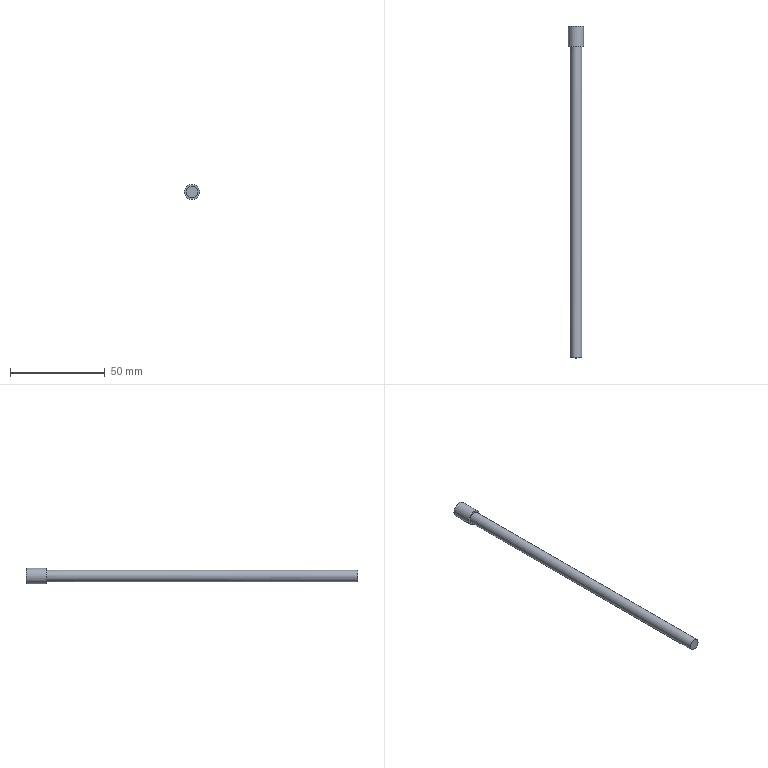Part | NX | features solid 2 | 1 solid | 5 faces | box 8 x 175 x 8 mm | volume 5190 mm3 | plane 3 | cylinder 2 | commonest cylinder face diameters 6 x1 8 x1
STEP:
#1=CARTESIAN_POINT('',(-39.,-65.,-52.));
#2=VERTEX_POINT('',#1);
#3=CARTESIAN_POINT('',(-42.,-65.,-52.));
#4=DIRECTION('',(0.,1.,0.));
#5=DIRECTION('',(1.,0.,0.));
#6=AXIS2_PLACEMENT_3D('',#3,#4,#5);
#7=CIRCLE('',#6,3.);
#8=EDGE_CURVE('',#2,#2,#7,.T.);
#9=ORIENTED_EDGE('',*,*,#8,.F.);
#10=EDGE_LOOP('',(#9));
#11=FACE_BOUND('',#10,.T.);
#12=CARTESIAN_POINT('',(-42.,-65.,-52.));
#13=DIRECTION('',(0.,-1.,0.));
#14=DIRECTION('',(0.,0.,-1.));
#15=AXIS2_PLACEMENT_3D('',#12,#13,#14);
#16=PLANE('',#15);
#17=ADVANCED_FACE('',(#11),#16,.T.);
#18=CARTESIAN_POINT('',(-42.,99.,-55.));
#19=VERTEX_POINT('',#18);
#20=CARTESIAN_POINT('',(-42.,99.,-52.));
#21=DIRECTION('',(0.,-1.,0.));
#22=DIRECTION('',(0.,0.,-1.));
#23=AXIS2_PLACEMENT_3D('',#20,#21,#22);
#24=CIRCLE('',#23,3.);
#25=EDGE_CURVE('',#19,#19,#24,.F.);
#26=ORIENTED_EDGE('',*,*,#25,.F.);
#27=EDGE_LOOP('',(#26));
#28=FACE_BOUND('',#27,.T.);
#29=ORIENTED_EDGE('',*,*,#8,.T.);
#30=EDGE_LOOP('',(#29));
#31=FACE_BOUND('',#30,.T.);
#32=CARTESIAN_POINT('',(-42.,110.,-52.));
#33=DIRECTION('',(0.,-1.,0.));
#34=DIRECTION('',(1.,0.,0.));
#35=AXIS2_PLACEMENT_3D('',#32,#33,#34);
#36=CYLINDRICAL_SURFACE('',#35,3.);
#37=ADVANCED_FACE('',(#28,#31),#36,.T.);
#38=ORIENTED_EDGE('',*,*,#25,.T.);
#39=EDGE_LOOP('',(#38));
#40=FACE_BOUND('',#39,.T.);
#41=CARTESIAN_POINT('',(-38.,99.,-52.));
#42=VERTEX_POINT('',#41);
#43=CARTESIAN_POINT('',(-42.,99.,-52.));
#44=DIRECTION('',(0.,1.,0.));
#45=DIRECTION('',(1.,0.,0.));
#46=AXIS2_PLACEMENT_3D('',#43,#44,#45);
#47=CIRCLE('',#46,4.);
#48=EDGE_CURVE('',#42,#42,#47,.T.);
#49=ORIENTED_EDGE('',*,*,#48,.F.);
#50=EDGE_LOOP('',(#49));
#51=FACE_BOUND('',#50,.T.);
#52=CARTESIAN_POINT('',(-42.,99.,-52.));
#53=DIRECTION('',(0.,-1.,0.));
#54=DIRECTION('',(0.,0.,-1.));
#55=AXIS2_PLACEMENT_3D('',#52,#53,#54);
#56=PLANE('',#55);
#57=ADVANCED_FACE('',(#40,#51),#56,.T.);
#58=ORIENTED_EDGE('',*,*,#48,.T.);
#59=EDGE_LOOP('',(#58));
#60=FACE_BOUND('',#59,.T.);
#61=CARTESIAN_POINT('',(-38.,110.,-52.));
#62=VERTEX_POINT('',#61);
#63=CARTESIAN_POINT('',(-42.,110.,-52.));
#64=DIRECTION('',(0.,-1.,0.));
#65=DIRECTION('',(1.,0.,0.));
#66=AXIS2_PLACEMENT_3D('',#63,#64,#65);
#67=CIRCLE('',#66,4.);
#68=EDGE_CURVE('',#62,#62,#67,.T.);
#69=ORIENTED_EDGE('',*,*,#68,.T.);
#70=EDGE_LOOP('',(#69));
#71=FACE_BOUND('',#70,.T.);
#72=CARTESIAN_POINT('',(-42.,110.,-52.));
#73=DIRECTION('',(0.,-1.,0.));
#74=DIRECTION('',(1.,0.,0.));
#75=AXIS2_PLACEMENT_3D('',#72,#73,#74);
#76=CYLINDRICAL_SURFACE('',#75,4.);
#77=ADVANCED_FACE('',(#60,#71),#76,.T.);
#78=ORIENTED_EDGE('',*,*,#68,.F.);
#79=EDGE_LOOP('',(#78));
#80=FACE_BOUND('',#79,.T.);
#81=CARTESIAN_POINT('',(-42.,110.,-52.));
#82=DIRECTION('',(0.,1.,0.));
#83=DIRECTION('',(0.,0.,1.));
#84=AXIS2_PLACEMENT_3D('',#81,#82,#83);
#85=PLANE('',#84);
#86=ADVANCED_FACE('',(#80),#85,.T.);
#87=CLOSED_SHELL('',(#17,#37,#57,#77,#86));
#88=MANIFOLD_SOLID_BREP('',#87);
#89=(LENGTH_UNIT()NAMED_UNIT(*)SI_UNIT(.MILLI.,.METRE.));
#90=UNCERTAINTY_MEASURE_WITH_UNIT(LENGTH_MEASURE(0.00001),#89,'','');
#91=(NAMED_UNIT(*)PLANE_ANGLE_UNIT()SI_UNIT($,.RADIAN.));
#92=(NAMED_UNIT(*)SI_UNIT($,.STERADIAN.)SOLID_ANGLE_UNIT());
#93=(GEOMETRIC_REPRESENTATION_CONTEXT(3)GLOBAL_UNCERTAINTY_ASSIGNED_CONTEXT((#90))GLOBAL_UNIT_ASSIGNED_CONTEXT((#89,#91,#92))REPRESENTATION_CONTEXT('',''));
#94=ADVANCED_BREP_SHAPE_REPRESENTATION('',(#88),#93);